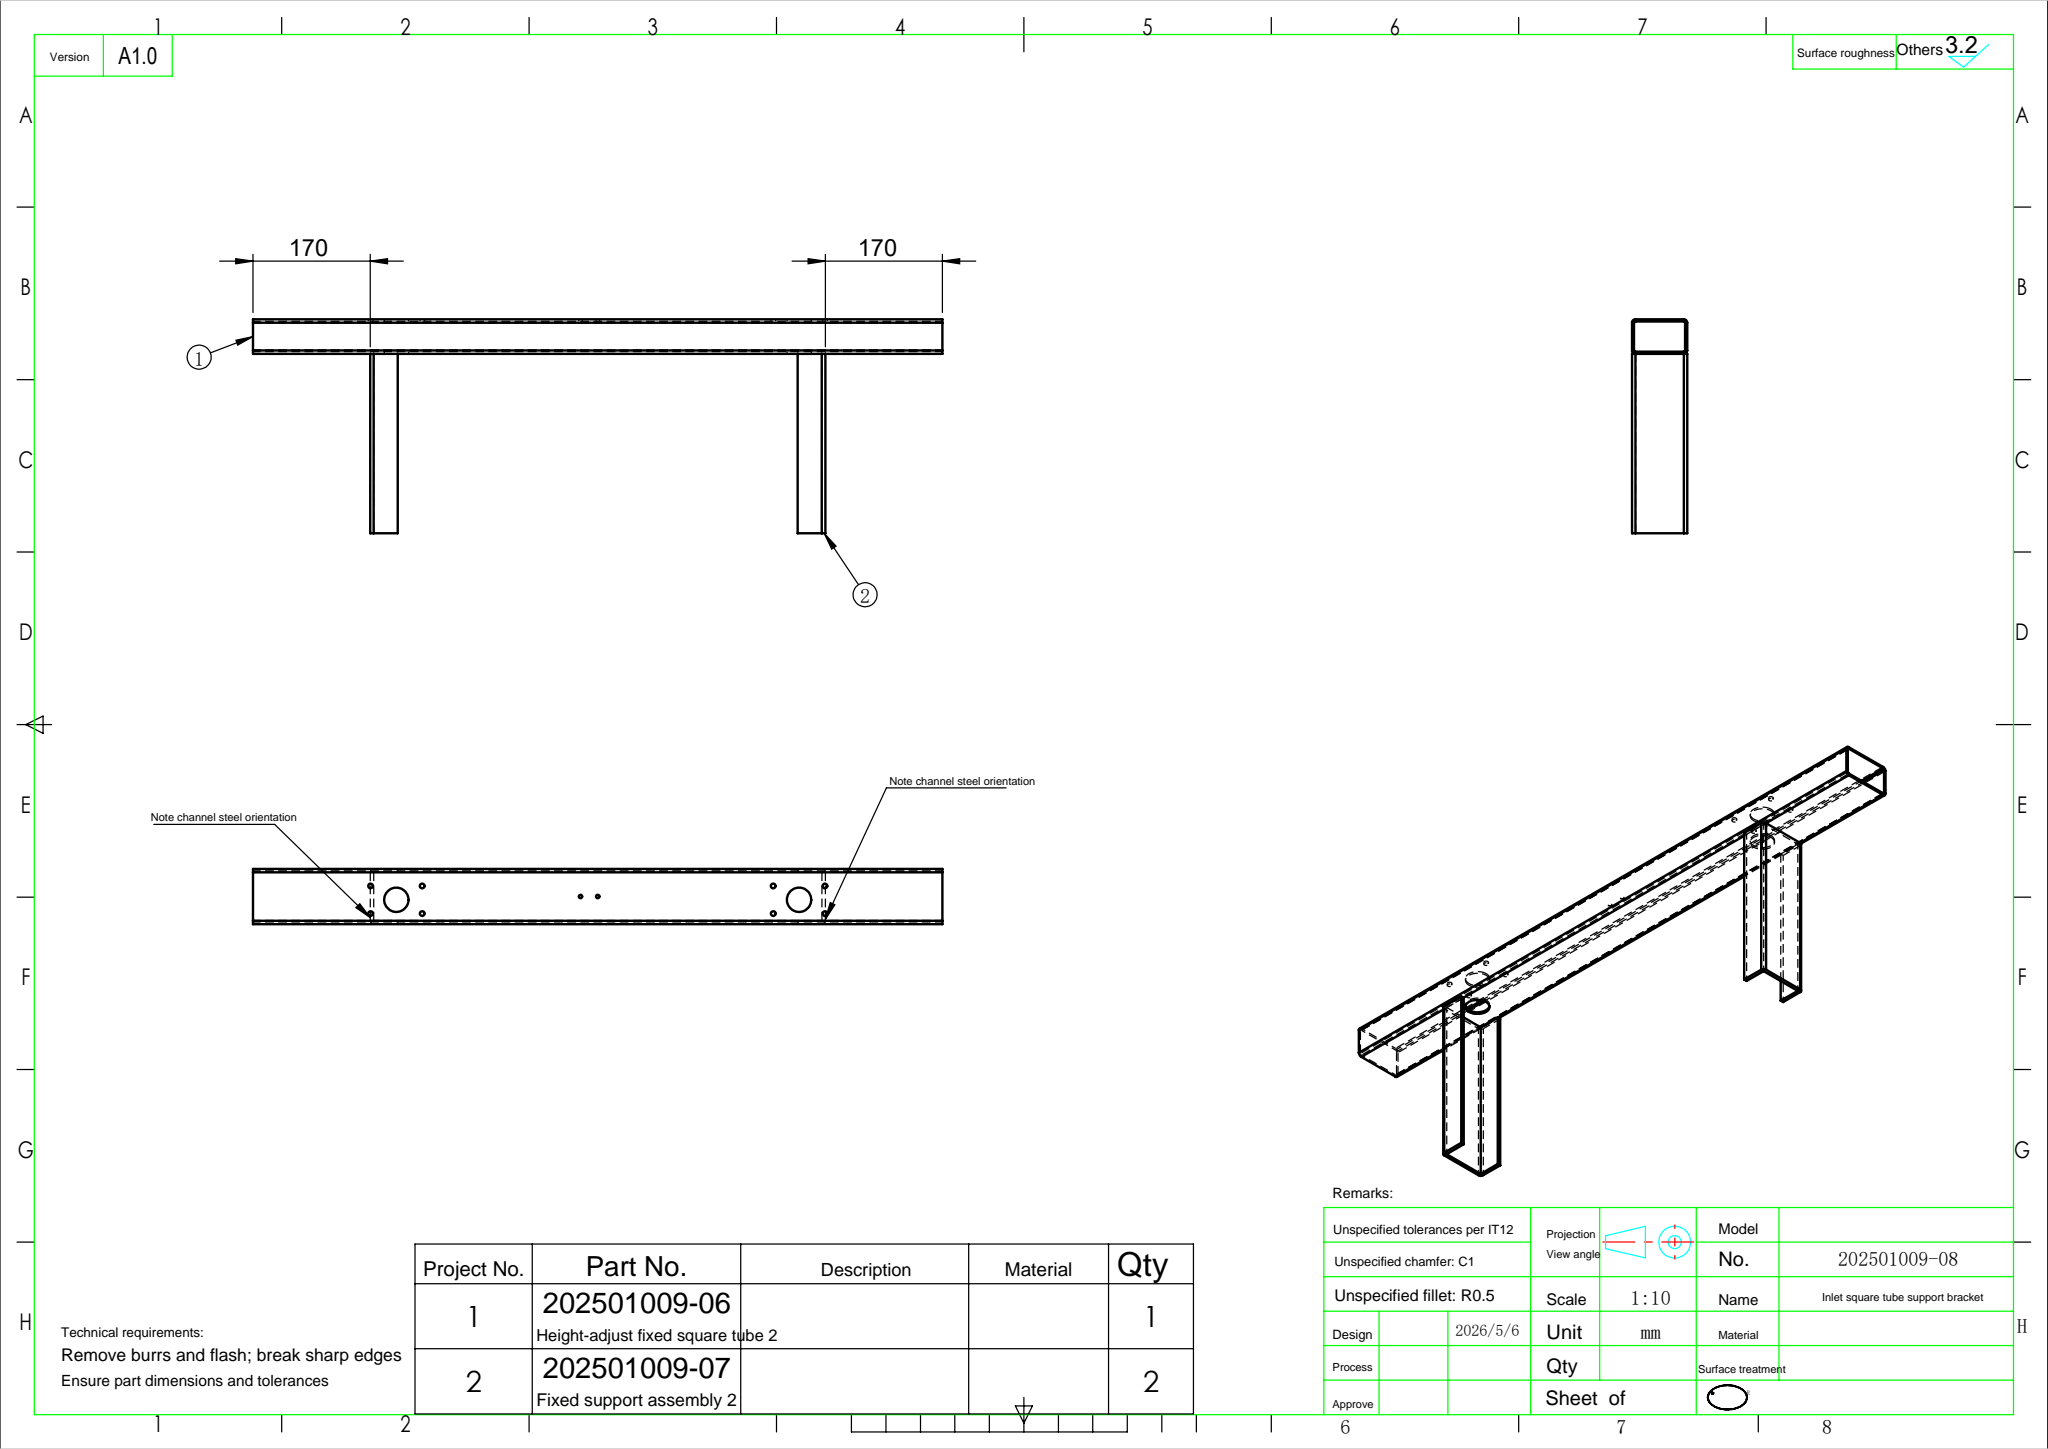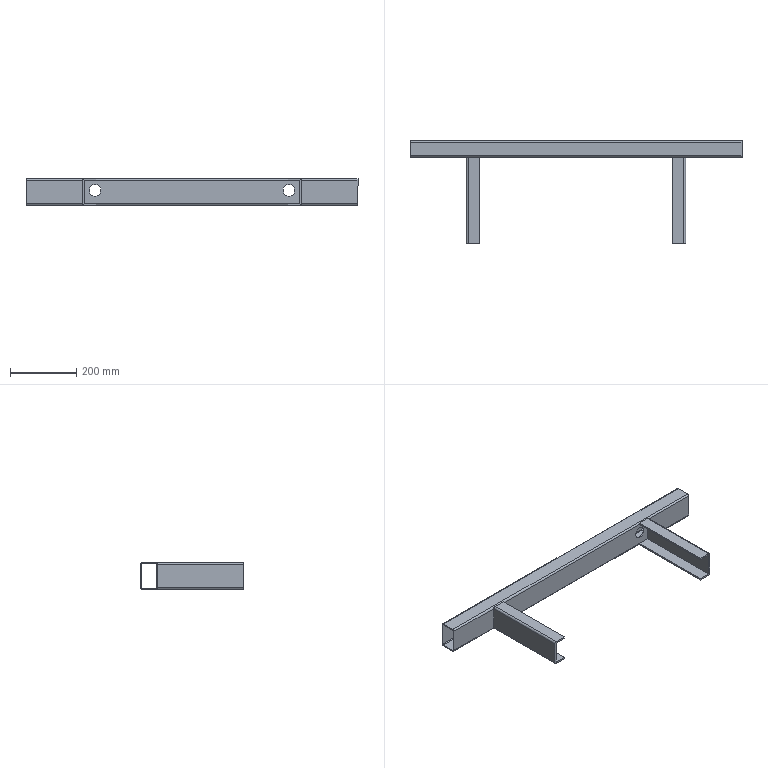Part | SolidWorks | 3 solids | 70 faces | box 1000 x 310 x 80 mm | volume 1097727 mm3 | cylinder 40 | plane 30 | commonest cylinder face diameters 6.8 x16 10 x8 35.2 x8 4 x4 5 x4